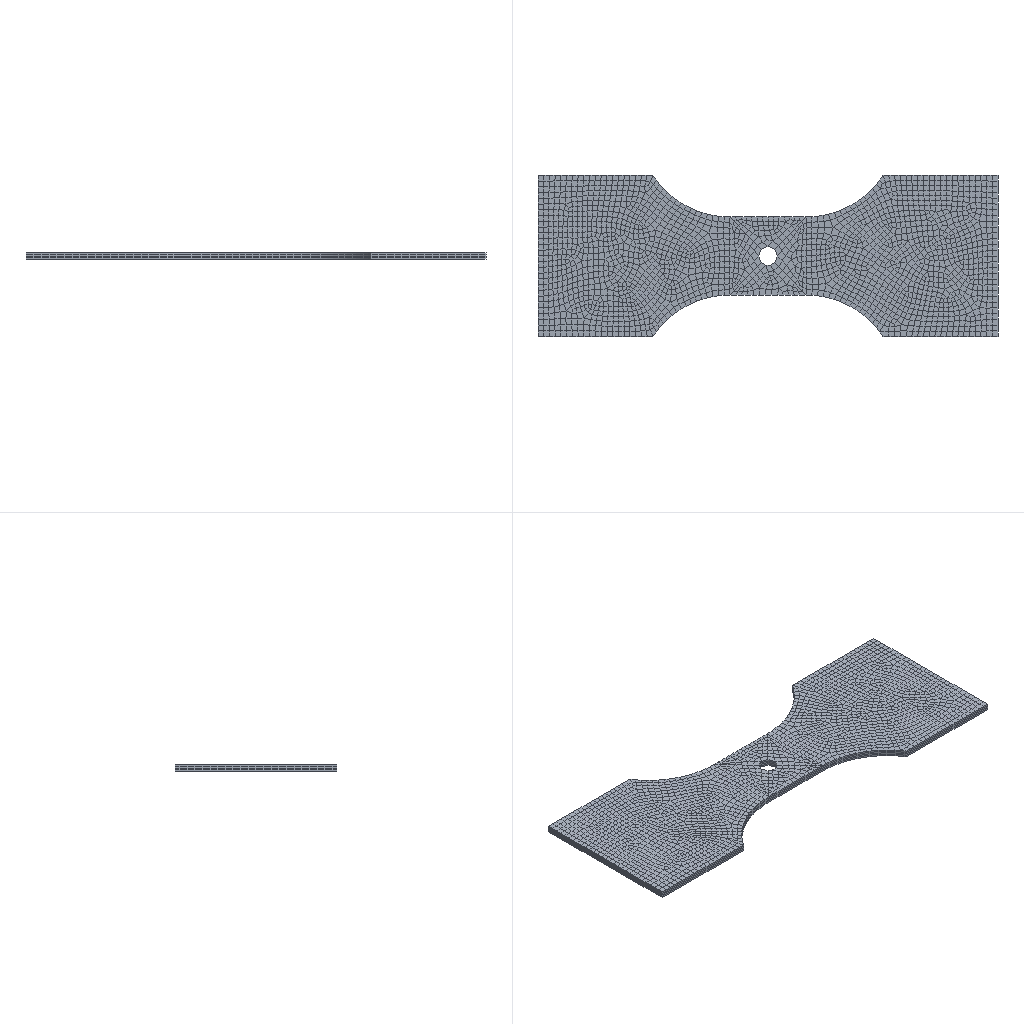Simulation study | abaqus
Set-up summary:
category,name,step,type,value,unit,region
solver,abaqus
solver,version,,,Abaqus/Standard 2020
units,not stated in the deck,,not stated
analysis,deck,,transient,transient
load_step,Step-1,Step-1,transient
load_step,requested,,,1
mesh,nodes,,,18320
mesh,elements,,,15204
element_type,C3D8R,,solid,8688
element_type,COH3D8,,cohesive,6516
load,load commands in deck,,count,1
bc,support commands in deck,,count,7
material,COH,,in results
material,MATERIAL-1,,in results
check,setup vs results,,match,"per instance, exact: element labels, types and connectivity; labels of the nodes the elements use; coordinates of those nodes at SINGLE_PRECISION in 1 of 1 instance(s)"
Abaqus input file, long lists of numbers shortened:
*Heading
** Job name: Job-1 Model name: Model-1
** Generated by: Abaqus/CAE 2020
*Preprint, echo=NO, model=NO, history=NO, contact=NO
**
** PARTS
**
*Part, name=partwork
*Node
      1,  -53.707,   14.773,           0.
      2,  -67.423,  0.7215,           0.
** (18318 more lines like these left out)
*Element, type=C3D8R
 1, 16031, 16034, 16033, 16032,   142,   143,  1507,  1505
 2, 16035, 16038, 16037, 16036,  1497,  1496,   160,   161
** (8686 more lines like these left out)
*Element, type=COH3D8
 8689,   247,  1673,  1671,   248, 11454, 11453, 11452, 11451
 8690,  1662,   257,   256,  1663, 11458, 11457, 11456, 11455
** (6514 more lines like these left out)
*Nset, nset=Set-8, generate
     1,  18320,      1
*Elset, elset=Set-8, generate
    1,  8688,     1
*Elset, elset=CohesiveSeam-1-Elements, generate
  8689,  15204,      1
*Nset, nset=CohesiveSeam-1-TopNodes, generate
 11451,  18320,      1
*Nset, nset=CohesiveSeam-1-BottomNodes
    1,    2,    3,    4,    5,   11,   12,   13,   14,   15,   21,   22,   23,   24,   25,   26
   27,   28,   29,   30,   36,   37,   38,   39,   40,   41,   42,   43,   44,   45,   51,   52
** (428 more lines like these left out)
*Elset, elset=__PickedSurf6_S1, internal, generate
  8689,  15204,      1
*Surface, type=ELEMENT, name=_PickedSurf6, internal
__PickedSurf6_S1, S1
*Elset, elset=_CohesiveSeam-1-TopSurf_S2, internal, generate
  8689,  15204,      1
*Surface, type=ELEMENT, name=CohesiveSeam-1-TopSurf
_CohesiveSeam-1-TopSurf_S2, S2
*Elset, elset=_CohesiveSeam-1-BottomSurf_S1, internal, generate
  8689,  15204,      1
*Surface, type=ELEMENT, name=CohesiveSeam-1-BottomSurf
_CohesiveSeam-1-BottomSurf_S1, S1
*Orientation, name=Ori-1
1., 0., 0., 0., 1., 0.
1, 0.
** Section: work
*Solid Section, elset=Set-8, orientation=Ori-1, material=Material-1
,
** Section: coh
*Cohesive Section, elset=CohesiveSeam-1-Elements, controls=EC-1, material=coh, response=TRACTION SEPARATION, thickness=SPECIFIED
0.001,
*End Part
**
**
** ASSEMBLY
**
*Assembly, name=Assembly
**
*Instance, name=partwork-1, part=partwork
*End Instance
**
*Nset, nset=Set-1, instance=partwork-1
     2,     3,     6,    10,    22,    23,    27,    28,    32,    33,    59,    60,    61,    62,    63,    64
    65,    66,    67,    68,    69,    70,    71,    72,    73,    74,    75,    76,    77,    78,   101,   102
** (515 more lines like these left out)
*Elset, elset=Set-1, instance=partwork-1
   633,   634,   635,   636,   637,   638,   639,   640,   641,   642,   643,   644,   645,   646,   647,   648
   649,   650,   651,   652,   653,   654,   655,   656,   657,   658,   659,   660,   661,   662,   663,   664
** (425 more lines like these left out)
*Nset, nset=Set-2, instance=partwork-1
    12,    13,    16,    20,    37,    38,    42,    43,    47,    48,    79,    80,    81,    82,    83,    84
    85,    86,    87,    88,    89,    90,    91,    92,    93,    94,    95,    96,    97,    98,   106,   107
** (512 more lines like these left out)
*Elset, elset=Set-2, instance=partwork-1
  3558,  3559,  3560,  3561,  3562,  3563,  3564,  3565,  3566,  3567,  3568,  3569,  3570,  3571,  3572,  3573
  3574,  3575,  3576,  3577,  3578,  3579,  3580,  3581,  3582,  3583,  3584,  3585,  3586,  3587,  3588,  3589
** (422 more lines like these left out)
*End Assembly
**
** ELEMENT CONTROLS
**
*Section Controls, name=EC-1, ELEMENT DELETION=YES, VISCOSITY=0.001
1., 1., 1.
*Amplitude, name=Amp-1
             0.,              0.,              1.,              1.
**
** MATERIALS
**
*Material, name=Material-1
*Density
 1e-09,
*Elastic, type=ENGINEERING CONSTANTS
 54.3, 54.3, 34.3,  0.4, 0.45, 0.42,  10.,  10.
   8.,
*Material, name=coh
*Damage Initiation, criterion=QUADE
 0.0001, 0.0001, 0.0001
*Damage Evolution, type=DISPLACEMENT
 1e-05,
*Damage Stabilization
0.001
*Density
 1e-09,
*Elastic, type=TRACTION
40.,3.,2.
** ----------------------------------------------------------------
**
** STEP: Step-1
**
*Step, name=Step-1, nlgeom=YES, inc=1000
*Dynamic
0.001,1.,1e-05
**
** BOUNDARY CONDITIONS
**
** Name: BC-1 Type: 对称/反对称/完全固定
*Boundary
Set-1, ENCASTRE
** Name: BC-2 Type: 位移/转角
*Boundary, amplitude=Amp-1
Set-2, 1, 1, 1.
Set-2, 2, 2
Set-2, 3, 3
Set-2, 4, 4
Set-2, 5, 5
Set-2, 6, 6
**
** OUTPUT REQUESTS
**
*Restart, write, number interval=1, time marks=NO
**
** FIELD OUTPUT: F-Output-1
**
*Output, field, frequency=1
*Node Output
A, RF, U, V
*Element Output, directions=YES
DAMAGEC, DAMAGEFC, DAMAGEFT, DAMAGEMC, DAMAGEMT, DAMAGET, E, HSNFCCRT, HSNFTCRT, HSNMCCRT, HSNMTCRT, LE, MISES, PE, PEEQ, S
SDEG, STATUS
*Contact Output
CDISP, CSTRESS
**
** HISTORY OUTPUT: H-Output-1
**
*Output, history, variable=PRESELECT, number interval=200, time marks=NO
*End Step
Results summary:
result,step,,partial,increments=37 time=0.01999/1.0
result,analysis,,,transient
result,last_loadstep,,,1
result,primary field,,,U
result,reaction total,,FX,0.000457,model units
result,reaction total,,FY,1.7e-05,model units
result,reaction total,,FZ,-1e-06,model units